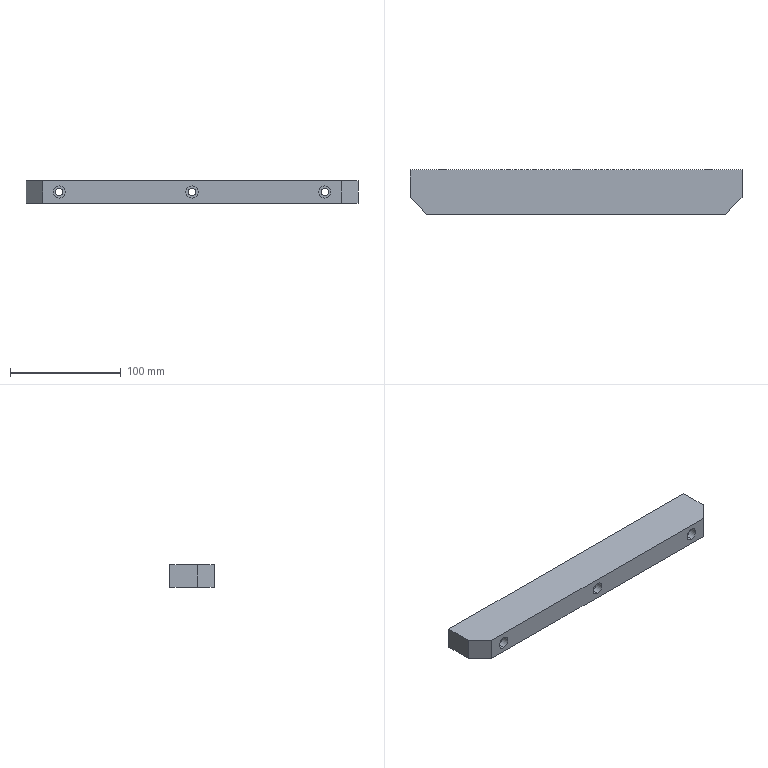Part | SolidWorks | features BaseBody 1 | 1 solid | 23 faces | box 300 x 40 x 20 mm | volume 230154 mm3 | cylinder 12 | plane 11 | commonest cylinder face diameters 6.6 x6 11 x6
STEP:
#1=CARTESIAN_POINT('',(-120.,6.8,5.5));
#2=VERTEX_POINT('',#1);
#3=CARTESIAN_POINT('',(-120.,6.8,-5.5));
#4=VERTEX_POINT('',#3);
#5=CARTESIAN_POINT('',(-120.,6.8,0.));
#6=DIRECTION('',(0.,-1.,0.));
#7=DIRECTION('',(0.,0.,-1.));
#8=AXIS2_PLACEMENT_3D('',#5,#6,#7);
#9=CIRCLE('',#8,5.5);
#10=EDGE_CURVE('',#2,#4,#9,.T.);
#11=ORIENTED_EDGE('',*,*,#10,.F.);
#12=CARTESIAN_POINT('',(-120.,0.,5.5));
#13=VERTEX_POINT('',#12);
#14=CARTESIAN_POINT('',(-120.,0.,5.5));
#15=DIRECTION('',(0.,-1.,0.));
#16=VECTOR('',#15,1000.);
#17=LINE('',#14,#16);
#18=EDGE_CURVE('',#2,#13,#17,.T.);
#19=ORIENTED_EDGE('',*,*,#18,.T.);
#20=CARTESIAN_POINT('',(-120.,0.,-5.5));
#21=VERTEX_POINT('',#20);
#22=CARTESIAN_POINT('',(-120.,0.,0.));
#23=DIRECTION('',(0.,-1.,0.));
#24=DIRECTION('',(0.,0.,-1.));
#25=AXIS2_PLACEMENT_3D('',#22,#23,#24);
#26=CIRCLE('',#25,5.5);
#27=EDGE_CURVE('',#13,#21,#26,.T.);
#28=ORIENTED_EDGE('',*,*,#27,.T.);
#29=CARTESIAN_POINT('',(-120.,0.,-5.5));
#30=DIRECTION('',(0.,-1.,0.));
#31=VECTOR('',#30,1000.);
#32=LINE('',#29,#31);
#33=EDGE_CURVE('',#4,#21,#32,.T.);
#34=ORIENTED_EDGE('',*,*,#33,.F.);
#35=EDGE_LOOP('',(#11,#19,#28,#34));
#36=FACE_OUTER_BOUND('',#35,.T.);
#37=CARTESIAN_POINT('',(-120.,0.,0.));
#38=DIRECTION('',(0.,-1.,0.));
#39=DIRECTION('',(0.,0.,-1.));
#40=AXIS2_PLACEMENT_3D('',#37,#38,#39);
#41=CYLINDRICAL_SURFACE('',#40,5.5);
#42=ADVANCED_FACE('',(#36),#41,.F.);
#43=CARTESIAN_POINT('',(-120.,40.,3.3));
#44=VERTEX_POINT('',#43);
#45=CARTESIAN_POINT('',(-120.,40.,-3.3));
#46=VERTEX_POINT('',#45);
#47=CARTESIAN_POINT('',(-120.,40.,0.));
#48=DIRECTION('',(0.,-1.,0.));
#49=DIRECTION('',(0.,0.,-1.));
#50=AXIS2_PLACEMENT_3D('',#47,#48,#49);
#51=CIRCLE('',#50,3.3);
#52=EDGE_CURVE('',#44,#46,#51,.T.);
#53=ORIENTED_EDGE('',*,*,#52,.F.);
#54=CARTESIAN_POINT('',(-120.,6.8,3.3));
#55=VERTEX_POINT('',#54);
#56=CARTESIAN_POINT('',(-120.,0.,3.3));
#57=DIRECTION('',(0.,-1.,0.));
#58=VECTOR('',#57,1000.);
#59=LINE('',#56,#58);
#60=EDGE_CURVE('',#44,#55,#59,.T.);
#61=ORIENTED_EDGE('',*,*,#60,.T.);
#62=CARTESIAN_POINT('',(-120.,6.8,-3.3));
#63=VERTEX_POINT('',#62);
#64=CARTESIAN_POINT('',(-120.,6.8,0.));
#65=DIRECTION('',(0.,-1.,0.));
#66=DIRECTION('',(0.,0.,-1.));
#67=AXIS2_PLACEMENT_3D('',#64,#65,#66);
#68=CIRCLE('',#67,3.3);
#69=EDGE_CURVE('',#55,#63,#68,.T.);
#70=ORIENTED_EDGE('',*,*,#69,.T.);
#71=CARTESIAN_POINT('',(-120.,0.,-3.3));
#72=DIRECTION('',(0.,-1.,0.));
#73=VECTOR('',#72,1000.);
#74=LINE('',#71,#73);
#75=EDGE_CURVE('',#46,#63,#74,.T.);
#76=ORIENTED_EDGE('',*,*,#75,.F.);
#77=EDGE_LOOP('',(#53,#61,#70,#76));
#78=FACE_OUTER_BOUND('',#77,.T.);
#79=CARTESIAN_POINT('',(-120.,0.,0.));
#80=DIRECTION('',(0.,-1.,0.));
#81=DIRECTION('',(0.,0.,-1.));
#82=AXIS2_PLACEMENT_3D('',#79,#80,#81);
#83=CYLINDRICAL_SURFACE('',#82,3.3);
#84=ADVANCED_FACE('',(#78),#83,.F.);
#85=CARTESIAN_POINT('',(0.,6.8,5.5));
#86=VERTEX_POINT('',#85);
#87=CARTESIAN_POINT('',(0.,6.8,-5.5));
#88=VERTEX_POINT('',#87);
#89=CARTESIAN_POINT('',(0.,6.8,0.));
#90=DIRECTION('',(0.,-1.,0.));
#91=DIRECTION('',(0.,0.,-1.));
#92=AXIS2_PLACEMENT_3D('',#89,#90,#91);
#93=CIRCLE('',#92,5.5);
#94=EDGE_CURVE('',#86,#88,#93,.T.);
#95=ORIENTED_EDGE('',*,*,#94,.F.);
#96=CARTESIAN_POINT('',(0.,0.,5.5));
#97=VERTEX_POINT('',#96);
#98=CARTESIAN_POINT('',(0.,0.,5.5));
#99=DIRECTION('',(0.,-1.,0.));
#100=VECTOR('',#99,1000.);
#101=LINE('',#98,#100);
#102=EDGE_CURVE('',#86,#97,#101,.T.);
#103=ORIENTED_EDGE('',*,*,#102,.T.);
#104=CARTESIAN_POINT('',(0.,0.,-5.5));
#105=VERTEX_POINT('',#104);
#106=CARTESIAN_POINT('',(0.,0.,0.));
#107=DIRECTION('',(0.,-1.,0.));
#108=DIRECTION('',(0.,0.,-1.));
#109=AXIS2_PLACEMENT_3D('',#106,#107,#108);
#110=CIRCLE('',#109,5.5);
#111=EDGE_CURVE('',#97,#105,#110,.T.);
#112=ORIENTED_EDGE('',*,*,#111,.T.);
#113=CARTESIAN_POINT('',(0.,0.,-5.5));
#114=DIRECTION('',(0.,-1.,0.));
#115=VECTOR('',#114,1000.);
#116=LINE('',#113,#115);
#117=EDGE_CURVE('',#88,#105,#116,.T.);
#118=ORIENTED_EDGE('',*,*,#117,.F.);
#119=EDGE_LOOP('',(#95,#103,#112,#118));
#120=FACE_OUTER_BOUND('',#119,.T.);
#121=CARTESIAN_POINT('',(0.,0.,0.));
#122=DIRECTION('',(0.,-1.,0.));
#123=DIRECTION('',(0.,0.,-1.));
#124=AXIS2_PLACEMENT_3D('',#121,#122,#123);
#125=CYLINDRICAL_SURFACE('',#124,5.5);
#126=ADVANCED_FACE('',(#120),#125,.F.);
#127=CARTESIAN_POINT('',(0.,40.,3.3));
#128=VERTEX_POINT('',#127);
#129=CARTESIAN_POINT('',(0.,40.,-3.3));
#130=VERTEX_POINT('',#129);
#131=CARTESIAN_POINT('',(0.,40.,0.));
#132=DIRECTION('',(0.,-1.,0.));
#133=DIRECTION('',(0.,0.,-1.));
#134=AXIS2_PLACEMENT_3D('',#131,#132,#133);
#135=CIRCLE('',#134,3.3);
#136=EDGE_CURVE('',#128,#130,#135,.T.);
#137=ORIENTED_EDGE('',*,*,#136,.F.);
#138=CARTESIAN_POINT('',(0.,6.8,3.3));
#139=VERTEX_POINT('',#138);
#140=CARTESIAN_POINT('',(0.,0.,3.3));
#141=DIRECTION('',(0.,-1.,0.));
#142=VECTOR('',#141,1000.);
#143=LINE('',#140,#142);
#144=EDGE_CURVE('',#128,#139,#143,.T.);
#145=ORIENTED_EDGE('',*,*,#144,.T.);
#146=CARTESIAN_POINT('',(0.,6.8,-3.3));
#147=VERTEX_POINT('',#146);
#148=CARTESIAN_POINT('',(0.,6.8,0.));
#149=DIRECTION('',(0.,-1.,0.));
#150=DIRECTION('',(0.,0.,-1.));
#151=AXIS2_PLACEMENT_3D('',#148,#149,#150);
#152=CIRCLE('',#151,3.3);
#153=EDGE_CURVE('',#139,#147,#152,.T.);
#154=ORIENTED_EDGE('',*,*,#153,.T.);
#155=CARTESIAN_POINT('',(0.,0.,-3.3));
#156=DIRECTION('',(0.,-1.,0.));
#157=VECTOR('',#156,1000.);
#158=LINE('',#155,#157);
#159=EDGE_CURVE('',#130,#147,#158,.T.);
#160=ORIENTED_EDGE('',*,*,#159,.F.);
#161=EDGE_LOOP('',(#137,#145,#154,#160));
#162=FACE_OUTER_BOUND('',#161,.T.);
#163=CARTESIAN_POINT('',(0.,0.,0.));
#164=DIRECTION('',(0.,-1.,0.));
#165=DIRECTION('',(0.,0.,-1.));
#166=AXIS2_PLACEMENT_3D('',#163,#164,#165);
#167=CYLINDRICAL_SURFACE('',#166,3.3);
#168=ADVANCED_FACE('',(#162),#167,.F.);
#169=CARTESIAN_POINT('',(120.,6.8,5.5));
#170=VERTEX_POINT('',#169);
#171=CARTESIAN_POINT('',(120.,6.8,-5.5));
#172=VERTEX_POINT('',#171);
#173=CARTESIAN_POINT('',(120.,6.8,0.));
#174=DIRECTION('',(0.,-1.,0.));
#175=DIRECTION('',(0.,0.,-1.));
#176=AXIS2_PLACEMENT_3D('',#173,#174,#175);
#177=CIRCLE('',#176,5.5);
#178=EDGE_CURVE('',#170,#172,#177,.T.);
#179=ORIENTED_EDGE('',*,*,#178,.F.);
#180=CARTESIAN_POINT('',(120.,0.,5.5));
#181=VERTEX_POINT('',#180);
#182=CARTESIAN_POINT('',(120.,0.,5.5));
#183=DIRECTION('',(0.,-1.,0.));
#184=VECTOR('',#183,1000.);
#185=LINE('',#182,#184);
#186=EDGE_CURVE('',#170,#181,#185,.T.);
#187=ORIENTED_EDGE('',*,*,#186,.T.);
#188=CARTESIAN_POINT('',(120.,0.,-5.5));
#189=VERTEX_POINT('',#188);
#190=CARTESIAN_POINT('',(120.,0.,0.));
#191=DIRECTION('',(0.,-1.,0.));
#192=DIRECTION('',(0.,0.,-1.));
#193=AXIS2_PLACEMENT_3D('',#190,#191,#192);
#194=CIRCLE('',#193,5.5);
#195=EDGE_CURVE('',#181,#189,#194,.T.);
#196=ORIENTED_EDGE('',*,*,#195,.T.);
#197=CARTESIAN_POINT('',(120.,0.,-5.5));
#198=DIRECTION('',(0.,-1.,0.));
#199=VECTOR('',#198,1000.);
#200=LINE('',#197,#199);
#201=EDGE_CURVE('',#172,#189,#200,.T.);
#202=ORIENTED_EDGE('',*,*,#201,.F.);
#203=EDGE_LOOP('',(#179,#187,#196,#202));
#204=FACE_OUTER_BOUND('',#203,.T.);
#205=CARTESIAN_POINT('',(120.,0.,0.));
#206=DIRECTION('',(0.,-1.,0.));
#207=DIRECTION('',(0.,0.,-1.));
#208=AXIS2_PLACEMENT_3D('',#205,#206,#207);
#209=CYLINDRICAL_SURFACE('',#208,5.5);
#210=ADVANCED_FACE('',(#204),#209,.F.);
#211=CARTESIAN_POINT('',(120.,40.,3.3));
#212=VERTEX_POINT('',#211);
#213=CARTESIAN_POINT('',(120.,40.,-3.3));
#214=VERTEX_POINT('',#213);
#215=CARTESIAN_POINT('',(120.,40.,0.));
#216=DIRECTION('',(0.,-1.,0.));
#217=DIRECTION('',(0.,0.,-1.));
#218=AXIS2_PLACEMENT_3D('',#215,#216,#217);
#219=CIRCLE('',#218,3.3);
#220=EDGE_CURVE('',#212,#214,#219,.T.);
#221=ORIENTED_EDGE('',*,*,#220,.F.);
#222=CARTESIAN_POINT('',(120.,6.8,3.3));
#223=VERTEX_POINT('',#222);
#224=CARTESIAN_POINT('',(120.,0.,3.3));
#225=DIRECTION('',(0.,-1.,0.));
#226=VECTOR('',#225,1000.);
#227=LINE('',#224,#226);
#228=EDGE_CURVE('',#212,#223,#227,.T.);
#229=ORIENTED_EDGE('',*,*,#228,.T.);
#230=CARTESIAN_POINT('',(120.,6.8,-3.3));
#231=VERTEX_POINT('',#230);
#232=CARTESIAN_POINT('',(120.,6.8,0.));
#233=DIRECTION('',(0.,-1.,0.));
#234=DIRECTION('',(0.,0.,-1.));
#235=AXIS2_PLACEMENT_3D('',#232,#233,#234);
#236=CIRCLE('',#235,3.3);
#237=EDGE_CURVE('',#223,#231,#236,.T.);
#238=ORIENTED_EDGE('',*,*,#237,.T.);
#239=CARTESIAN_POINT('',(120.,0.,-3.3));
#240=DIRECTION('',(0.,-1.,0.));
#241=VECTOR('',#240,1000.);
#242=LINE('',#239,#241);
#243=EDGE_CURVE('',#214,#231,#242,.T.);
#244=ORIENTED_EDGE('',*,*,#243,.F.);
#245=EDGE_LOOP('',(#221,#229,#238,#244));
#246=FACE_OUTER_BOUND('',#245,.T.);
#247=CARTESIAN_POINT('',(120.,0.,0.));
#248=DIRECTION('',(0.,-1.,0.));
#249=DIRECTION('',(0.,0.,-1.));
#250=AXIS2_PLACEMENT_3D('',#247,#248,#249);
#251=CYLINDRICAL_SURFACE('',#250,3.3);
#252=ADVANCED_FACE('',(#246),#251,.F.);
#253=CARTESIAN_POINT('',(-135.,0.,-10.));
#254=VERTEX_POINT('',#253);
#255=CARTESIAN_POINT('',(-150.,15.,-10.));
#256=VERTEX_POINT('',#255);
#257=CARTESIAN_POINT('',(-150.,15.,-10.));
#258=DIRECTION('',(-0.7071,0.7071,0.));
#259=VECTOR('',#258,1000.);
#260=LINE('',#257,#259);
#261=EDGE_CURVE('',#254,#256,#260,.T.);
#262=ORIENTED_EDGE('',*,*,#261,.F.);
#263=CARTESIAN_POINT('',(-135.,0.,10.));
#264=VERTEX_POINT('',#263);
#265=CARTESIAN_POINT('',(-135.,0.,-10.));
#266=DIRECTION('',(0.,0.,-1.));
#267=VECTOR('',#266,1000.);
#268=LINE('',#265,#267);
#269=EDGE_CURVE('',#264,#254,#268,.T.);
#270=ORIENTED_EDGE('',*,*,#269,.F.);
#271=CARTESIAN_POINT('',(-150.,15.,10.));
#272=VERTEX_POINT('',#271);
#273=CARTESIAN_POINT('',(-150.,15.,10.));
#274=DIRECTION('',(0.7071,-0.7071,0.));
#275=VECTOR('',#274,1000.);
#276=LINE('',#273,#275);
#277=EDGE_CURVE('',#272,#264,#276,.T.);
#278=ORIENTED_EDGE('',*,*,#277,.F.);
#279=CARTESIAN_POINT('',(-150.,15.,10.));
#280=DIRECTION('',(0.,0.,1.));
#281=VECTOR('',#280,1000.);
#282=LINE('',#279,#281);
#283=EDGE_CURVE('',#256,#272,#282,.T.);
#284=ORIENTED_EDGE('',*,*,#283,.F.);
#285=EDGE_LOOP('',(#262,#270,#278,#284));
#286=FACE_OUTER_BOUND('',#285,.T.);
#287=CARTESIAN_POINT('',(-150.,15.,10.));
#288=DIRECTION('',(-0.7071,-0.7071,0.));
#289=DIRECTION('',(-0.7071,0.7071,0.));
#290=AXIS2_PLACEMENT_3D('',#287,#288,#289);
#291=PLANE('',#290);
#292=ADVANCED_FACE('',(#286),#291,.T.);
#293=CARTESIAN_POINT('',(135.,0.,10.));
#294=VERTEX_POINT('',#293);
#295=CARTESIAN_POINT('',(150.,15.,10.));
#296=VERTEX_POINT('',#295);
#297=CARTESIAN_POINT('',(150.,15.,10.));
#298=DIRECTION('',(0.7071,0.7071,0.));
#299=VECTOR('',#298,1000.);
#300=LINE('',#297,#299);
#301=EDGE_CURVE('',#294,#296,#300,.T.);
#302=ORIENTED_EDGE('',*,*,#301,.F.);
#303=CARTESIAN_POINT('',(135.,0.,-10.));
#304=VERTEX_POINT('',#303);
#305=CARTESIAN_POINT('',(135.,0.,10.));
#306=DIRECTION('',(0.,0.,1.));
#307=VECTOR('',#306,1000.);
#308=LINE('',#305,#307);
#309=EDGE_CURVE('',#304,#294,#308,.T.);
#310=ORIENTED_EDGE('',*,*,#309,.F.);
#311=CARTESIAN_POINT('',(150.,15.,-10.));
#312=VERTEX_POINT('',#311);
#313=CARTESIAN_POINT('',(150.,15.,-10.));
#314=DIRECTION('',(-0.7071,-0.7071,0.));
#315=VECTOR('',#314,1000.);
#316=LINE('',#313,#315);
#317=EDGE_CURVE('',#312,#304,#316,.T.);
#318=ORIENTED_EDGE('',*,*,#317,.F.);
#319=CARTESIAN_POINT('',(150.,15.,-10.));
#320=DIRECTION('',(0.,0.,-1.));
#321=VECTOR('',#320,1000.);
#322=LINE('',#319,#321);
#323=EDGE_CURVE('',#296,#312,#322,.T.);
#324=ORIENTED_EDGE('',*,*,#323,.F.);
#325=EDGE_LOOP('',(#302,#310,#318,#324));
#326=FACE_OUTER_BOUND('',#325,.T.);
#327=CARTESIAN_POINT('',(150.,15.,10.));
#328=DIRECTION('',(0.7071,-0.7071,0.));
#329=DIRECTION('',(0.,0.,-1.));
#330=AXIS2_PLACEMENT_3D('',#327,#328,#329);
#331=PLANE('',#330);
#332=ADVANCED_FACE('',(#326),#331,.T.);
#333=CARTESIAN_POINT('',(-120.,6.8,0.));
#334=DIRECTION('',(0.,-1.,0.));
#335=DIRECTION('',(0.,0.,-1.));
#336=AXIS2_PLACEMENT_3D('',#333,#334,#335);
#337=CIRCLE('',#336,3.3);
#338=EDGE_CURVE('',#63,#55,#337,.T.);
#339=ORIENTED_EDGE('',*,*,#338,.F.);
#340=ORIENTED_EDGE('',*,*,#69,.F.);
#341=EDGE_LOOP('',(#339,#340));
#342=FACE_BOUND('',#341,.T.);
#343=CARTESIAN_POINT('',(-120.,6.8,0.));
#344=DIRECTION('',(0.,-1.,0.));
#345=DIRECTION('',(0.,0.,-1.));
#346=AXIS2_PLACEMENT_3D('',#343,#344,#345);
#347=CIRCLE('',#346,5.5);
#348=EDGE_CURVE('',#4,#2,#347,.T.);
#349=ORIENTED_EDGE('',*,*,#348,.T.);
#350=ORIENTED_EDGE('',*,*,#10,.T.);
#351=EDGE_LOOP('',(#349,#350));
#352=FACE_OUTER_BOUND('',#351,.T.);
#353=CARTESIAN_POINT('',(-116.7,6.8,0.));
#354=DIRECTION('',(0.,1.,0.));
#355=DIRECTION('',(1.,0.,0.));
#356=AXIS2_PLACEMENT_3D('',#353,#354,#355);
#357=PLANE('',#356);
#358=ADVANCED_FACE('',(#342,#352),#357,.F.);
#359=CARTESIAN_POINT('',(0.,6.8,0.));
#360=DIRECTION('',(0.,-1.,0.));
#361=DIRECTION('',(0.,0.,-1.));
#362=AXIS2_PLACEMENT_3D('',#359,#360,#361);
#363=CIRCLE('',#362,3.3);
#364=EDGE_CURVE('',#147,#139,#363,.T.);
#365=ORIENTED_EDGE('',*,*,#364,.F.);
#366=ORIENTED_EDGE('',*,*,#153,.F.);
#367=EDGE_LOOP('',(#365,#366));
#368=FACE_BOUND('',#367,.T.);
#369=CARTESIAN_POINT('',(0.,6.8,0.));
#370=DIRECTION('',(0.,-1.,0.));
#371=DIRECTION('',(0.,0.,-1.));
#372=AXIS2_PLACEMENT_3D('',#369,#370,#371);
#373=CIRCLE('',#372,5.5);
#374=EDGE_CURVE('',#88,#86,#373,.T.);
#375=ORIENTED_EDGE('',*,*,#374,.T.);
#376=ORIENTED_EDGE('',*,*,#94,.T.);
#377=EDGE_LOOP('',(#375,#376));
#378=FACE_OUTER_BOUND('',#377,.T.);
#379=CARTESIAN_POINT('',(3.3,6.8,0.));
#380=DIRECTION('',(0.,1.,0.));
#381=DIRECTION('',(1.,0.,0.));
#382=AXIS2_PLACEMENT_3D('',#379,#380,#381);
#383=PLANE('',#382);
#384=ADVANCED_FACE('',(#368,#378),#383,.F.);
#385=CARTESIAN_POINT('',(120.,6.8,0.));
#386=DIRECTION('',(0.,-1.,0.));
#387=DIRECTION('',(0.,0.,-1.));
#388=AXIS2_PLACEMENT_3D('',#385,#386,#387);
#389=CIRCLE('',#388,3.3);
#390=EDGE_CURVE('',#231,#223,#389,.T.);
#391=ORIENTED_EDGE('',*,*,#390,.F.);
#392=ORIENTED_EDGE('',*,*,#237,.F.);
#393=EDGE_LOOP('',(#391,#392));
#394=FACE_BOUND('',#393,.T.);
#395=CARTESIAN_POINT('',(120.,6.8,0.));
#396=DIRECTION('',(0.,-1.,0.));
#397=DIRECTION('',(0.,0.,-1.));
#398=AXIS2_PLACEMENT_3D('',#395,#396,#397);
#399=CIRCLE('',#398,5.5);
#400=EDGE_CURVE('',#172,#170,#399,.T.);
#401=ORIENTED_EDGE('',*,*,#400,.T.);
#402=ORIENTED_EDGE('',*,*,#178,.T.);
#403=EDGE_LOOP('',(#401,#402));
#404=FACE_OUTER_BOUND('',#403,.T.);
#405=CARTESIAN_POINT('',(123.3,6.8,0.));
#406=DIRECTION('',(0.,1.,0.));
#407=DIRECTION('',(1.,0.,0.));
#408=AXIS2_PLACEMENT_3D('',#405,#406,#407);
#409=PLANE('',#408);
#410=ADVANCED_FACE('',(#394,#404),#409,.F.);
#411=CARTESIAN_POINT('',(120.,0.,0.));
#412=DIRECTION('',(0.,-1.,0.));
#413=DIRECTION('',(0.,0.,-1.));
#414=AXIS2_PLACEMENT_3D('',#411,#412,#413);
#415=CIRCLE('',#414,5.5);
#416=EDGE_CURVE('',#189,#181,#415,.T.);
#417=ORIENTED_EDGE('',*,*,#416,.F.);
#418=ORIENTED_EDGE('',*,*,#195,.F.);
#419=EDGE_LOOP('',(#417,#418));
#420=FACE_BOUND('',#419,.T.);
#421=CARTESIAN_POINT('',(0.,0.,0.));
#422=DIRECTION('',(0.,-1.,0.));
#423=DIRECTION('',(0.,0.,-1.));
#424=AXIS2_PLACEMENT_3D('',#421,#422,#423);
#425=CIRCLE('',#424,5.5);
#426=EDGE_CURVE('',#105,#97,#425,.T.);
#427=ORIENTED_EDGE('',*,*,#426,.F.);
#428=ORIENTED_EDGE('',*,*,#111,.F.);
#429=EDGE_LOOP('',(#427,#428));
#430=FACE_BOUND('',#429,.T.);
#431=CARTESIAN_POINT('',(-120.,0.,0.));
#432=DIRECTION('',(0.,-1.,0.));
#433=DIRECTION('',(0.,0.,-1.));
#434=AXIS2_PLACEMENT_3D('',#431,#432,#433);
#435=CIRCLE('',#434,5.5);
#436=EDGE_CURVE('',#21,#13,#435,.T.);
#437=ORIENTED_EDGE('',*,*,#436,.F.);
#438=ORIENTED_EDGE('',*,*,#27,.F.);
#439=EDGE_LOOP('',(#437,#438));
#440=FACE_BOUND('',#439,.T.);
#441=CARTESIAN_POINT('',(-150.,0.,-10.));
#442=DIRECTION('',(-1.,0.,0.));
#443=VECTOR('',#442,1000.);
#444=LINE('',#441,#443);
#445=EDGE_CURVE('',#304,#254,#444,.T.);
#446=ORIENTED_EDGE('',*,*,#445,.F.);
#447=ORIENTED_EDGE('',*,*,#309,.T.);
#448=CARTESIAN_POINT('',(-150.,0.,10.));
#449=DIRECTION('',(1.,0.,0.));
#450=VECTOR('',#449,1000.);
#451=LINE('',#448,#450);
#452=EDGE_CURVE('',#264,#294,#451,.T.);
#453=ORIENTED_EDGE('',*,*,#452,.F.);
#454=ORIENTED_EDGE('',*,*,#269,.T.);
#455=EDGE_LOOP('',(#446,#447,#453,#454));
#456=FACE_OUTER_BOUND('',#455,.T.);
#457=CARTESIAN_POINT('',(0.,0.,0.));
#458=DIRECTION('',(0.,-1.,0.));
#459=DIRECTION('',(0.,0.,-1.));
#460=AXIS2_PLACEMENT_3D('',#457,#458,#459);
#461=PLANE('',#460);
#462=ADVANCED_FACE('',(#420,#430,#440,#456),#461,.T.);
#463=CARTESIAN_POINT('',(120.,40.,0.));
#464=DIRECTION('',(0.,-1.,0.));
#465=DIRECTION('',(0.,0.,-1.));
#466=AXIS2_PLACEMENT_3D('',#463,#464,#465);
#467=CIRCLE('',#466,3.3);
#468=EDGE_CURVE('',#214,#212,#467,.T.);
#469=ORIENTED_EDGE('',*,*,#468,.T.);
#470=ORIENTED_EDGE('',*,*,#220,.T.);
#471=EDGE_LOOP('',(#469,#470));
#472=FACE_BOUND('',#471,.T.);
#473=CARTESIAN_POINT('',(0.,40.,0.));
#474=DIRECTION('',(0.,-1.,0.));
#475=DIRECTION('',(0.,0.,-1.));
#476=AXIS2_PLACEMENT_3D('',#473,#474,#475);
#477=CIRCLE('',#476,3.3);
#478=EDGE_CURVE('',#130,#128,#477,.T.);
#479=ORIENTED_EDGE('',*,*,#478,.T.);
#480=ORIENTED_EDGE('',*,*,#136,.T.);
#481=EDGE_LOOP('',(#479,#480));
#482=FACE_BOUND('',#481,.T.);
#483=CARTESIAN_POINT('',(-120.,40.,0.));
#484=DIRECTION('',(0.,-1.,0.));
#485=DIRECTION('',(0.,0.,-1.));
#486=AXIS2_PLACEMENT_3D('',#483,#484,#485);
#487=CIRCLE('',#486,3.3);
#488=EDGE_CURVE('',#46,#44,#487,.T.);
#489=ORIENTED_EDGE('',*,*,#488,.T.);
#490=ORIENTED_EDGE('',*,*,#52,.T.);
#491=EDGE_LOOP('',(#489,#490));
#492=FACE_BOUND('',#491,.T.);
#493=CARTESIAN_POINT('',(150.,40.,10.));
#494=VERTEX_POINT('',#493);
#495=CARTESIAN_POINT('',(150.,40.,-10.));
#496=VERTEX_POINT('',#495);
#497=CARTESIAN_POINT('',(150.,40.,10.));
#498=DIRECTION('',(0.,0.,-1.));
#499=VECTOR('',#498,1000.);
#500=LINE('',#497,#499);
#501=EDGE_CURVE('',#494,#496,#500,.T.);
#502=ORIENTED_EDGE('',*,*,#501,.T.);
#503=CARTESIAN_POINT('',(-150.,40.,-10.));
#504=VERTEX_POINT('',#503);
#505=CARTESIAN_POINT('',(-150.,40.,-10.));
#506=DIRECTION('',(-1.,0.,0.));
#507=VECTOR('',#506,1000.);
#508=LINE('',#505,#507);
#509=EDGE_CURVE('',#496,#504,#508,.T.);
#510=ORIENTED_EDGE('',*,*,#509,.T.);
#511=CARTESIAN_POINT('',(-150.,40.,10.));
#512=VERTEX_POINT('',#511);
#513=CARTESIAN_POINT('',(-150.,40.,10.));
#514=DIRECTION('',(0.,0.,1.));
#515=VECTOR('',#514,1000.);
#516=LINE('',#513,#515);
#517=EDGE_CURVE('',#504,#512,#516,.T.);
#518=ORIENTED_EDGE('',*,*,#517,.T.);
#519=CARTESIAN_POINT('',(-150.,40.,10.));
#520=DIRECTION('',(1.,0.,0.));
#521=VECTOR('',#520,1000.);
#522=LINE('',#519,#521);
#523=EDGE_CURVE('',#512,#494,#522,.T.);
#524=ORIENTED_EDGE('',*,*,#523,.T.);
#525=EDGE_LOOP('',(#502,#510,#518,#524));
#526=FACE_OUTER_BOUND('',#525,.T.);
#527=CARTESIAN_POINT('',(0.,40.,0.));
#528=DIRECTION('',(0.,-1.,0.));
#529=DIRECTION('',(0.,0.,-1.));
#530=AXIS2_PLACEMENT_3D('',#527,#528,#529);
#531=PLANE('',#530);
#532=ADVANCED_FACE('',(#472,#482,#492,#526),#531,.F.);
#533=ORIENTED_EDGE('',*,*,#452,.T.);
#534=ORIENTED_EDGE('',*,*,#301,.T.);
#535=CARTESIAN_POINT('',(150.,40.,10.));
#536=DIRECTION('',(0.,-1.,0.));
#537=VECTOR('',#536,1000.);
#538=LINE('',#535,#537);
#539=EDGE_CURVE('',#494,#296,#538,.T.);
#540=ORIENTED_EDGE('',*,*,#539,.F.);
#541=ORIENTED_EDGE('',*,*,#523,.F.);
#542=CARTESIAN_POINT('',(-150.,40.,10.));
#543=DIRECTION('',(0.,-1.,0.));
#544=VECTOR('',#543,1000.);
#545=LINE('',#542,#544);
#546=EDGE_CURVE('',#512,#272,#545,.T.);
#547=ORIENTED_EDGE('',*,*,#546,.T.);
#548=ORIENTED_EDGE('',*,*,#277,.T.);
#549=EDGE_LOOP('',(#533,#534,#540,#541,#547,#548));
#550=FACE_OUTER_BOUND('',#549,.T.);
#551=CARTESIAN_POINT('',(-150.,40.,10.));
#552=DIRECTION('',(0.,0.,-1.));
#553=DIRECTION('',(0.,-1.,0.));
#554=AXIS2_PLACEMENT_3D('',#551,#552,#553);
#555=PLANE('',#554);
#556=ADVANCED_FACE('',(#550),#555,.F.);
#557=CARTESIAN_POINT('',(-150.,40.,-10.));
#558=DIRECTION('',(0.,-1.,0.));
#559=VECTOR('',#558,1000.);
#560=LINE('',#557,#559);
#561=EDGE_CURVE('',#504,#256,#560,.T.);
#562=ORIENTED_EDGE('',*,*,#561,.T.);
#563=ORIENTED_EDGE('',*,*,#283,.T.);
#564=ORIENTED_EDGE('',*,*,#546,.F.);
#565=ORIENTED_EDGE('',*,*,#517,.F.);
#566=EDGE_LOOP('',(#562,#563,#564,#565));
#567=FACE_OUTER_BOUND('',#566,.T.);
#568=CARTESIAN_POINT('',(-150.,40.,10.));
#569=DIRECTION('',(1.,0.,0.));
#570=DIRECTION('',(0.,1.,0.));
#571=AXIS2_PLACEMENT_3D('',#568,#569,#570);
#572=PLANE('',#571);
#573=ADVANCED_FACE('',(#567),#572,.F.);
#574=CARTESIAN_POINT('',(150.,40.,-10.));
#575=DIRECTION('',(0.,-1.,0.));
#576=VECTOR('',#575,1000.);
#577=LINE('',#574,#576);
#578=EDGE_CURVE('',#496,#312,#577,.T.);
#579=ORIENTED_EDGE('',*,*,#578,.T.);
#580=ORIENTED_EDGE('',*,*,#317,.T.);
#581=ORIENTED_EDGE('',*,*,#445,.T.);
#582=ORIENTED_EDGE('',*,*,#261,.T.);
#583=ORIENTED_EDGE('',*,*,#561,.F.);
#584=ORIENTED_EDGE('',*,*,#509,.F.);
#585=EDGE_LOOP('',(#579,#580,#581,#582,#583,#584));
#586=FACE_OUTER_BOUND('',#585,.T.);
#587=CARTESIAN_POINT('',(-150.,40.,-10.));
#588=DIRECTION('',(0.,0.,1.));
#589=DIRECTION('',(1.,0.,0.));
#590=AXIS2_PLACEMENT_3D('',#587,#588,#589);
#591=PLANE('',#590);
#592=ADVANCED_FACE('',(#586),#591,.F.);
#593=ORIENTED_EDGE('',*,*,#539,.T.);
#594=ORIENTED_EDGE('',*,*,#323,.T.);
#595=ORIENTED_EDGE('',*,*,#578,.F.);
#596=ORIENTED_EDGE('',*,*,#501,.F.);
#597=EDGE_LOOP('',(#593,#594,#595,#596));
#598=FACE_OUTER_BOUND('',#597,.T.);
#599=CARTESIAN_POINT('',(150.,40.,10.));
#600=DIRECTION('',(-1.,0.,0.));
#601=DIRECTION('',(0.,0.,1.));
#602=AXIS2_PLACEMENT_3D('',#599,#600,#601);
#603=PLANE('',#602);
#604=ADVANCED_FACE('',(#598),#603,.F.);
#605=ORIENTED_EDGE('',*,*,#228,.F.);
#606=ORIENTED_EDGE('',*,*,#468,.F.);
#607=ORIENTED_EDGE('',*,*,#243,.T.);
#608=ORIENTED_EDGE('',*,*,#390,.T.);
#609=EDGE_LOOP('',(#605,#606,#607,#608));
#610=FACE_OUTER_BOUND('',#609,.T.);
#611=CARTESIAN_POINT('',(120.,0.,0.));
#612=DIRECTION('',(0.,-1.,0.));
#613=DIRECTION('',(0.,0.,-1.));
#614=AXIS2_PLACEMENT_3D('',#611,#612,#613);
#615=CYLINDRICAL_SURFACE('',#614,3.3);
#616=ADVANCED_FACE('',(#610),#615,.F.);
#617=ORIENTED_EDGE('',*,*,#186,.F.);
#618=ORIENTED_EDGE('',*,*,#400,.F.);
#619=ORIENTED_EDGE('',*,*,#201,.T.);
#620=ORIENTED_EDGE('',*,*,#416,.T.);
#621=EDGE_LOOP('',(#617,#618,#619,#620));
#622=FACE_OUTER_BOUND('',#621,.T.);
#623=CARTESIAN_POINT('',(120.,0.,0.));
#624=DIRECTION('',(0.,-1.,0.));
#625=DIRECTION('',(0.,0.,-1.));
#626=AXIS2_PLACEMENT_3D('',#623,#624,#625);
#627=CYLINDRICAL_SURFACE('',#626,5.5);
#628=ADVANCED_FACE('',(#622),#627,.F.);
#629=ORIENTED_EDGE('',*,*,#144,.F.);
#630=ORIENTED_EDGE('',*,*,#478,.F.);
#631=ORIENTED_EDGE('',*,*,#159,.T.);
#632=ORIENTED_EDGE('',*,*,#364,.T.);
#633=EDGE_LOOP('',(#629,#630,#631,#632));
#634=FACE_OUTER_BOUND('',#633,.T.);
#635=CARTESIAN_POINT('',(0.,0.,0.));
#636=DIRECTION('',(0.,-1.,0.));
#637=DIRECTION('',(0.,0.,-1.));
#638=AXIS2_PLACEMENT_3D('',#635,#636,#637);
#639=CYLINDRICAL_SURFACE('',#638,3.3);
#640=ADVANCED_FACE('',(#634),#639,.F.);
#641=ORIENTED_EDGE('',*,*,#102,.F.);
#642=ORIENTED_EDGE('',*,*,#374,.F.);
#643=ORIENTED_EDGE('',*,*,#117,.T.);
#644=ORIENTED_EDGE('',*,*,#426,.T.);
#645=EDGE_LOOP('',(#641,#642,#643,#644));
#646=FACE_OUTER_BOUND('',#645,.T.);
#647=CARTESIAN_POINT('',(0.,0.,0.));
#648=DIRECTION('',(0.,-1.,0.));
#649=DIRECTION('',(0.,0.,-1.));
#650=AXIS2_PLACEMENT_3D('',#647,#648,#649);
#651=CYLINDRICAL_SURFACE('',#650,5.5);
#652=ADVANCED_FACE('',(#646),#651,.F.);
#653=ORIENTED_EDGE('',*,*,#60,.F.);
#654=ORIENTED_EDGE('',*,*,#488,.F.);
#655=ORIENTED_EDGE('',*,*,#75,.T.);
#656=ORIENTED_EDGE('',*,*,#338,.T.);
#657=EDGE_LOOP('',(#653,#654,#655,#656));
#658=FACE_OUTER_BOUND('',#657,.T.);
#659=CARTESIAN_POINT('',(-120.,0.,0.));
#660=DIRECTION('',(0.,-1.,0.));
#661=DIRECTION('',(0.,0.,-1.));
#662=AXIS2_PLACEMENT_3D('',#659,#660,#661);
#663=CYLINDRICAL_SURFACE('',#662,3.3);
#664=ADVANCED_FACE('',(#658),#663,.F.);
#665=ORIENTED_EDGE('',*,*,#18,.F.);
#666=ORIENTED_EDGE('',*,*,#348,.F.);
#667=ORIENTED_EDGE('',*,*,#33,.T.);
#668=ORIENTED_EDGE('',*,*,#436,.T.);
#669=EDGE_LOOP('',(#665,#666,#667,#668));
#670=FACE_OUTER_BOUND('',#669,.T.);
#671=CARTESIAN_POINT('',(-120.,0.,0.));
#672=DIRECTION('',(0.,-1.,0.));
#673=DIRECTION('',(0.,0.,-1.));
#674=AXIS2_PLACEMENT_3D('',#671,#672,#673);
#675=CYLINDRICAL_SURFACE('',#674,5.5);
#676=ADVANCED_FACE('',(#670),#675,.F.);
#677=CLOSED_SHELL('',(#42,#84,#126,#168,#210,#252,#292,#332,#358,#384,#410,#462,#532,#556,#573,#592,#604,#616,#628,#640,#652,#664,#676));
#678=MANIFOLD_SOLID_BREP('',#677);
#679=CARTESIAN_POINT('',(0.,0.,0.));
#680=DIRECTION('',(0.,0.,1.));
#681=DIRECTION('',(1.,0.,0.));
#682=AXIS2_PLACEMENT_3D('',#679,#680,#681);
#683=(LENGTH_UNIT()NAMED_UNIT(*)SI_UNIT(.MILLI.,.METRE.));
#684=UNCERTAINTY_MEASURE_WITH_UNIT(LENGTH_MEASURE(0.00001),#683,'','');
#685=(NAMED_UNIT(*)PLANE_ANGLE_UNIT()SI_UNIT($,.RADIAN.));
#686=(NAMED_UNIT(*)SI_UNIT($,.STERADIAN.)SOLID_ANGLE_UNIT());
#687=(GEOMETRIC_REPRESENTATION_CONTEXT(3)GLOBAL_UNCERTAINTY_ASSIGNED_CONTEXT((#684))GLOBAL_UNIT_ASSIGNED_CONTEXT((#683,#685,#686))REPRESENTATION_CONTEXT('',''));
#688=ADVANCED_BREP_SHAPE_REPRESENTATION('',(#678,#682),#687);